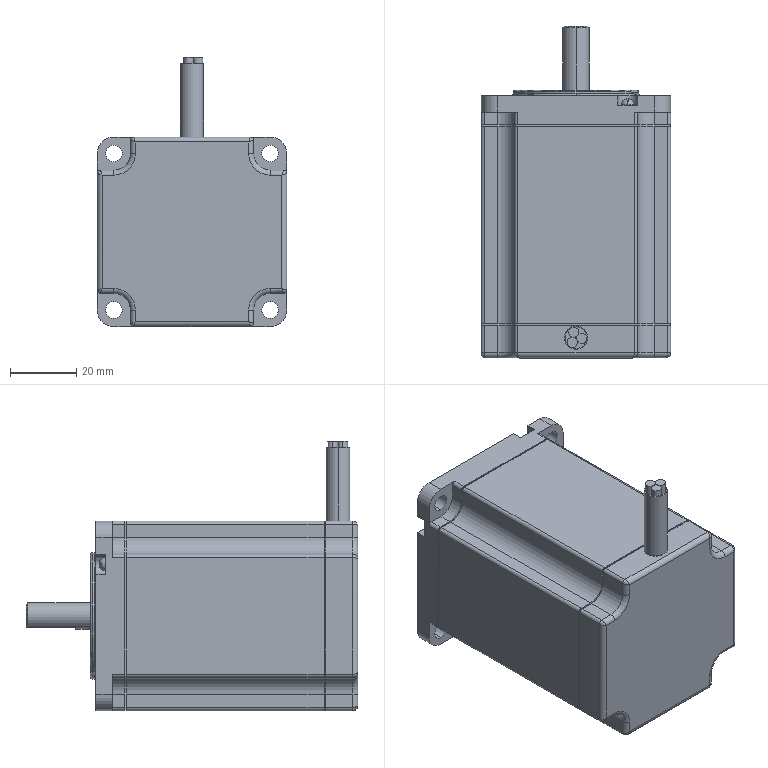Part | STEP file | 57系列三相混合式步进电机[573S15]大国工匠 | 4 solids | 254 faces | box 57.15 x 100 x 81.15 mm | volume 232236 mm3 | plane 131 | cylinder 97 | torus 16 | spline 8 | cone 2 | commonest cylinder face diameters 2 x24 10 x16 3 x12 4 x8 5 x8 11 x8